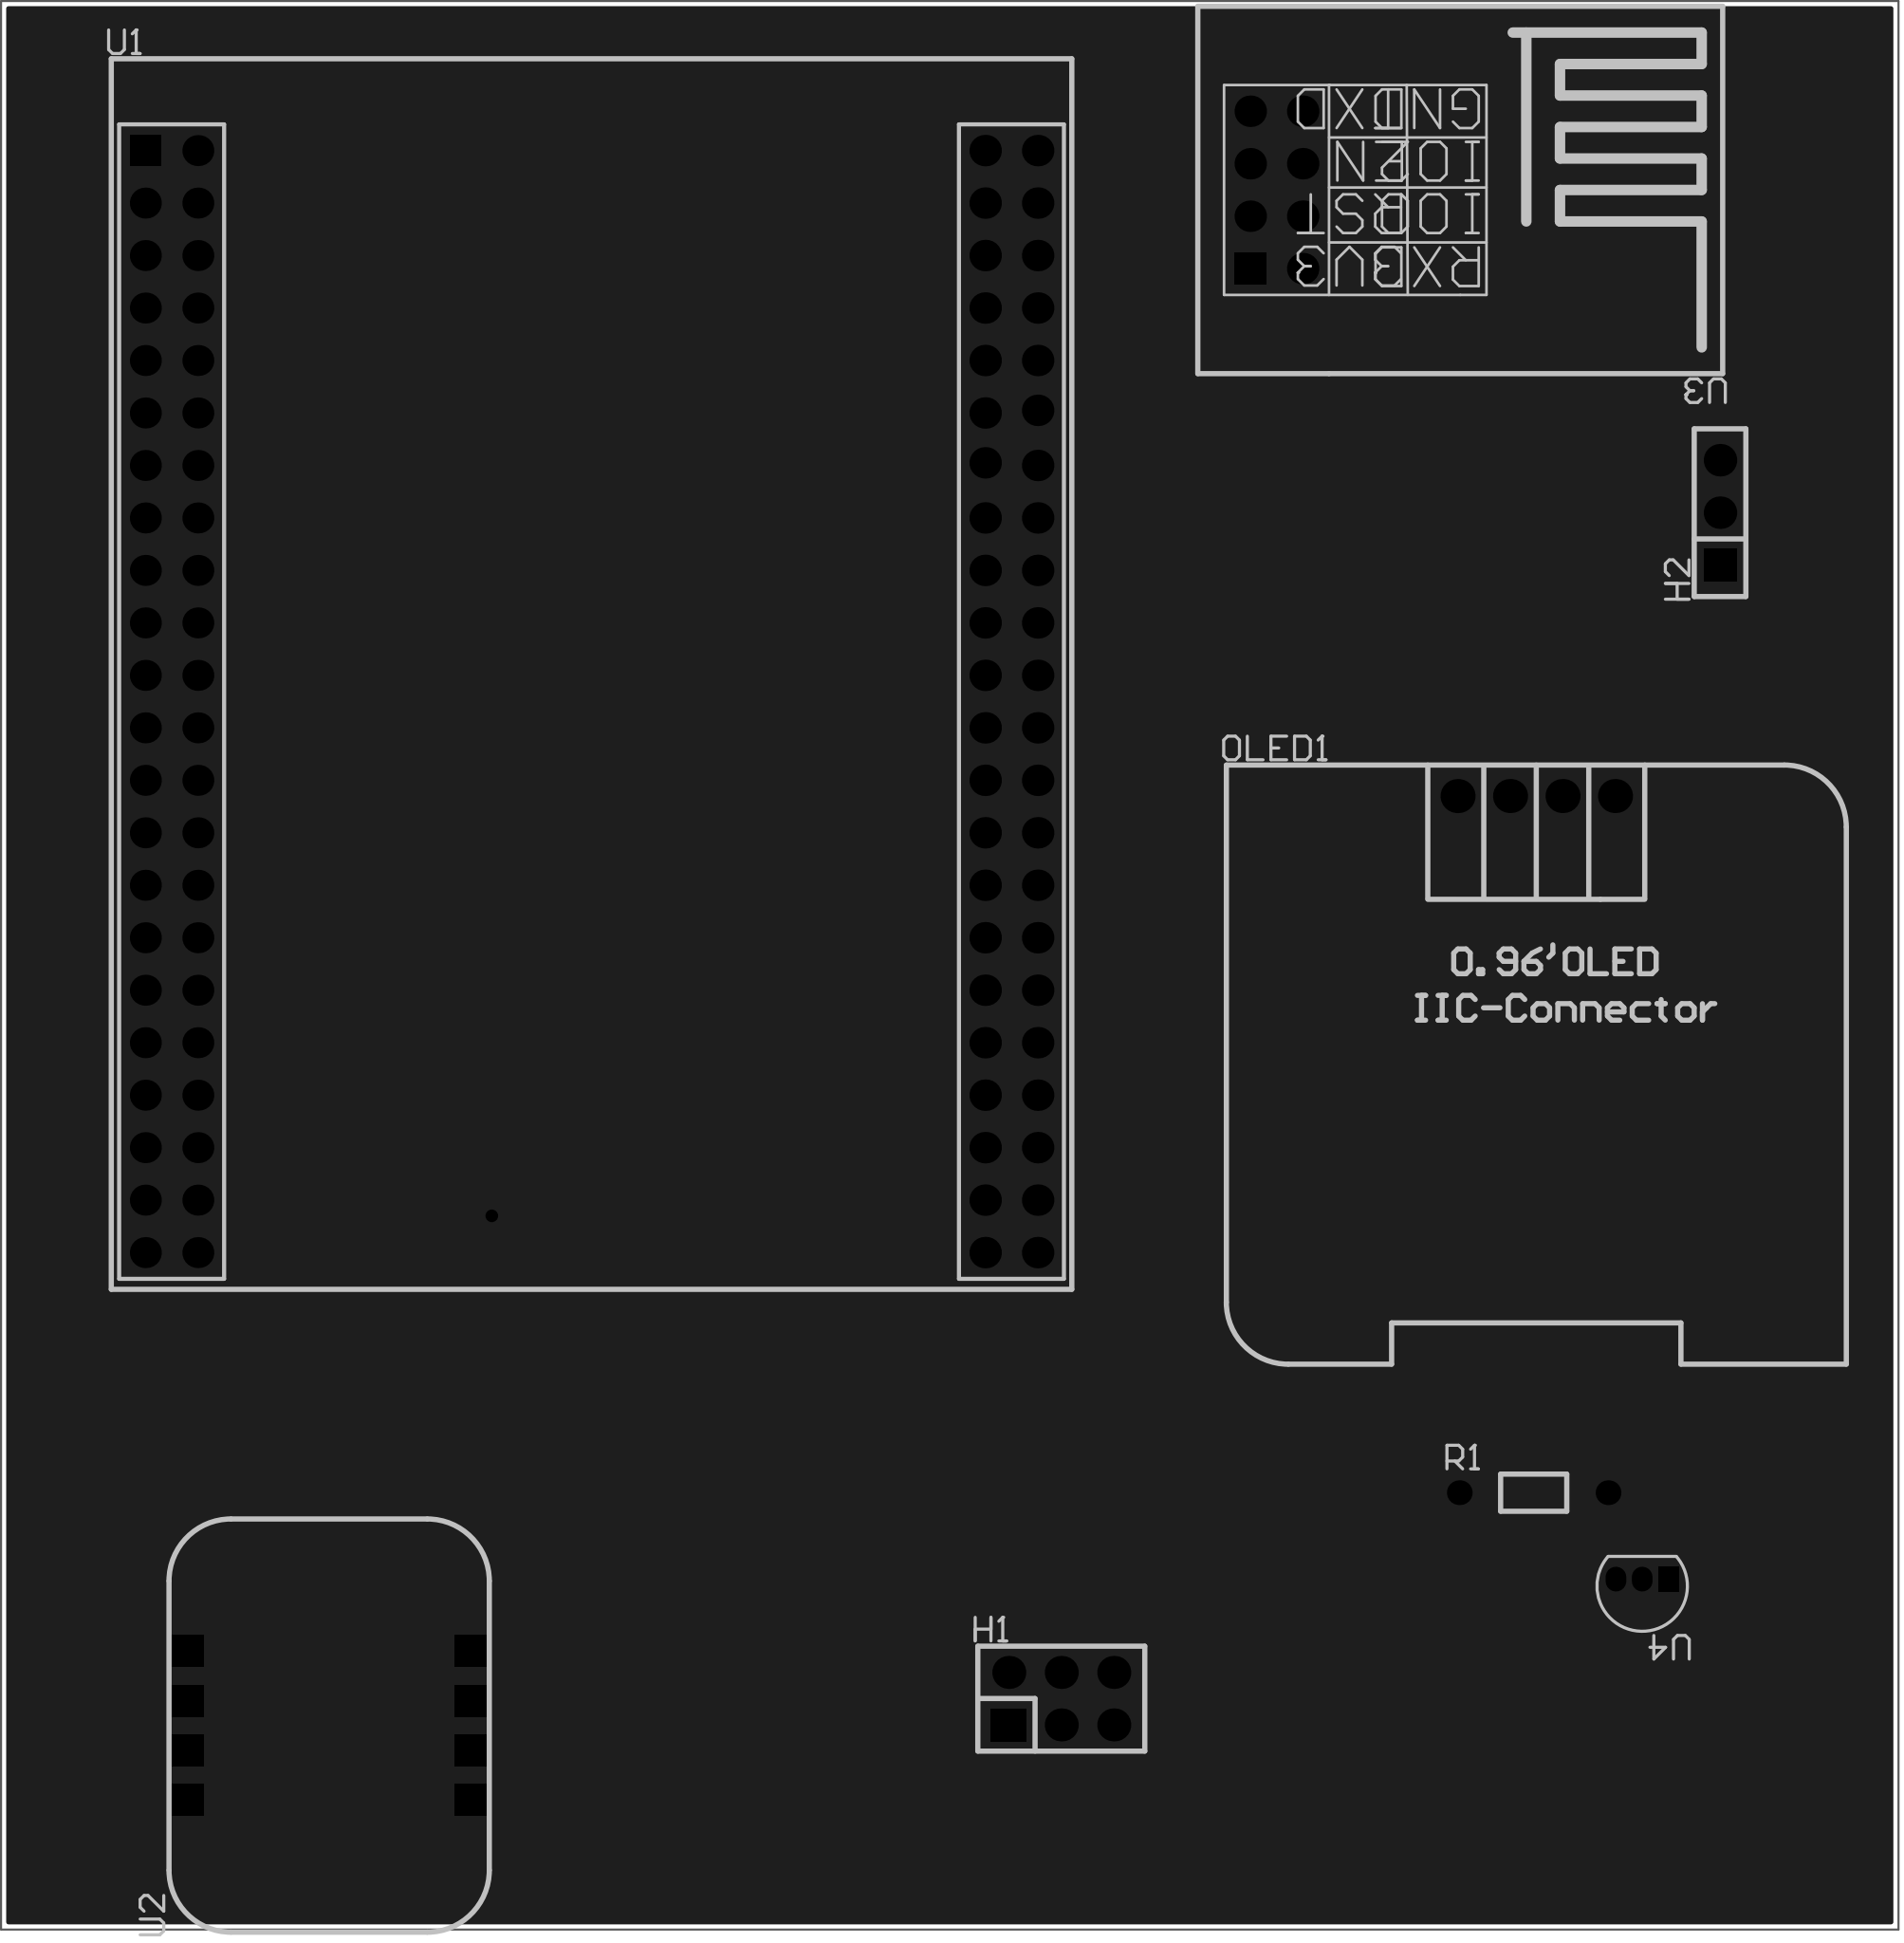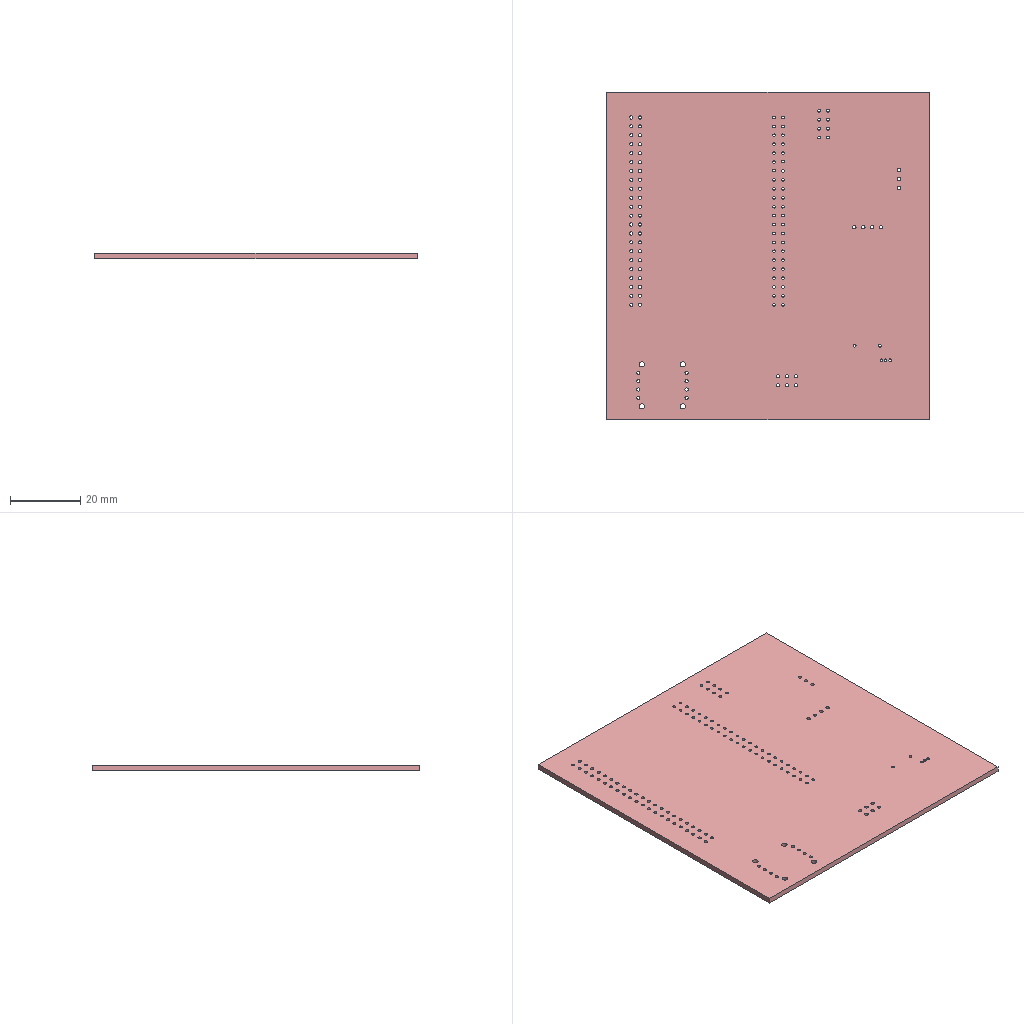Circuit board layout | Altium Designer | box 91.8 x 93.3 x 1.6 mm
Layer stack:
# Altium Designer layer stack of  (unit mm; dielectric type: 0 none, 1 core, 2 prepreg, 3 surface material)
index,name,kind,layer,copper_thickness_mm,dielectric_type,dielectric_thickness_mm,dielectric_material,dielectric_constant
0,Top Paste Mask Layer,other,,,,,,
1,Top Silkscreen Layer,other,,,,,,
2,Top Solder Mask Layer,dielectric,,,3,0.01,,3.3
3,Top Layer,copper,Top Layer,0.035,,,,
4,Dielectric1,dielectric,,,3,1.51,FR4,4.5
5,Bottom Layer,copper,Bottom Layer,0.035,,,,
6,Bottom Solder Mask Layer,dielectric,,,3,0.01,,3.3
7,Bottom Silkscreen Layer,other,,,,,,
8,Bottom Paste Mask Layer,other,,,,,,
# drill layer pairs: low layer,high layer
drill_pair,Top Layer,Bottom Layer
Part placement:
Designator,Comment,Layer,Footprint,Center-X(mm),Center-Y(mm),Rotation
H1,,TopLayer,HDR-TH_6P-P2.54-V-F-R2-C3-S2.54,141.605,98.552,0
H2,,TopLayer,HDR-TH_3P-P2.54-V-F,173.482,155.956,90
OLED1,,TopLayer,0.96OLED_4P,164.592,142.24,0
R1,4.7kΩ,TopLayer,Res_1/8W,164.465,108.521,0
U1,STM32F407VET6最小系统,TopLayer,STM32F407VET6最小系统,118.872,146.812,0
U2,MAX30102,TopLayer,MAX30102,106.172,97.249,90
U3,ESP01S,TopLayer,ESP01S,152.019,171.577,180
U4,DS18B20,TopLayer,TO-92-3_L4.5-W3.5-P1.27-L,169.715,104.338,180
Pad and via stacks:
# Altium Designer via and pad stacks of  (unit mm). Each distinct definition once, with the count of objects using it.
# via: kind,start_layer,end_layer,hole_mm,diameter_mm,mode(0 simple;1 top-mid-bottom;2 full stack),diameter_per_layer,count,example_net
# pad: kind,layer,hole_mm,hole_type(0 round;1 square;2 slot),plating,top_size,top_shape(1 round;2 rect;3 octagon;9 rounded rect),mid_size,bottom_size,mode,footprint,size_per_layer,count,example
pad,Multi-Layer,1,0,plated,1.7x1.6,2,1.7x1.6,1.7x1.6,0,HDR-TH_6P-P2.54-V-F-R2-C3-S2.54,,1,H1.1
pad,Multi-Layer,1,0,plated,1.6x1.6,1,1.6x1.6,1.6x1.6,0,HDR-TH_6P-P2.54-V-F-R2-C3-S2.54,,5,H1.2
pad,Multi-Layer,1.02,0,plated,1.575x1.575,1,1.575x1.575,1.575x1.575,0,HDR-TH_3P-P2.54-V-F,,2,H2.3
pad,Multi-Layer,1.02,0,plated,1.575x1.575,2,1.575x1.575,1.575x1.575,0,HDR-TH_3P-P2.54-V-F,,1,H2.1
pad,Multi-Layer,1,0,plated,1.65x1.65,1,1.65x1.65,1.65x1.65,0,0.96OLED_4P,,4,OLED1.4
pad,Multi-Layer,0.8001,0,plated,1.199x1.199,1,1.199x1.199,1.199x1.199,0,Res_1/8W,,2,R1.1
pad,Multi-Layer,0.9,0,plated,1.5x1.5,1,1.5x1.5,1.5x1.5,0,STM32F407VET6\u00D7\u00EE\u00D0\u00A1\u00CF\u00B5\u00CD\u00B3,,43,U1.4
pad,Multi-Layer,0.9,0,plated,1.5x1.5,2,1.5x1.5,1.5x1.5,0,STM32F407VET6\u00D7\u00EE\u00D0\u00A1\u00CF\u00B5\u00CD\u00B3,,1,U1.1
pad,Multi-Layer,0.762,2,plated,1.524x1.524,1,1.524x1.524,1.524x1.524,0,STM32F407VET6\u00D7\u00EE\u00D0\u00A1\u00CF\u00B5\u00CD\u00B3,,44,U1.45
pad,Multi-Layer,0.9144,0,plated,1.524x1.524,2,1.524x1.524,1.524x1.524,0,MAX30102,,8,U2.1
pad,Multi-Layer,0.81,0,plated,1.524x1.524,2,1.524x1.524,1.524x1.524,0,ESP01S,,1,U3.1
pad,Multi-Layer,0.81,0,plated,1.524x1.524,1,1.524x1.524,1.524x1.524,0,ESP01S,,7,U3.2
pad,Multi-Layer,0.7,2,plated,1x1.2,2,1x1.2,1x1.2,0,TO-92-3_L4.5-W3.5-P1.27-L,,1,U4.1
pad,Multi-Layer,0.7,2,plated,1x1.2,1,1x1.2,1x1.2,0,TO-92-3_L4.5-W3.5-P1.27-L,,2,U4.2
via,Top Layer,Bottom Layer,0.3048,0.61,0,,1,VCC
Copper pours:
name,layer,net,type(0 solid;1 hatched;2 none)
Top Layer-GND,Top Layer,GND,0
Bottom Layer-GND,Bottom Layer,GND,0
Design rules, without the lines most boards share:
# Altium Designer design rules of  (exported by Altium Designer, unit mm)
# columns: name | kind | enabled | priority | scope1 | scope2 | descriptor | typed fields (field=value)
creepage | 65 | enabled | 1 | All | All | Creepage Distance Constraint =(0mil) (All),(All) |